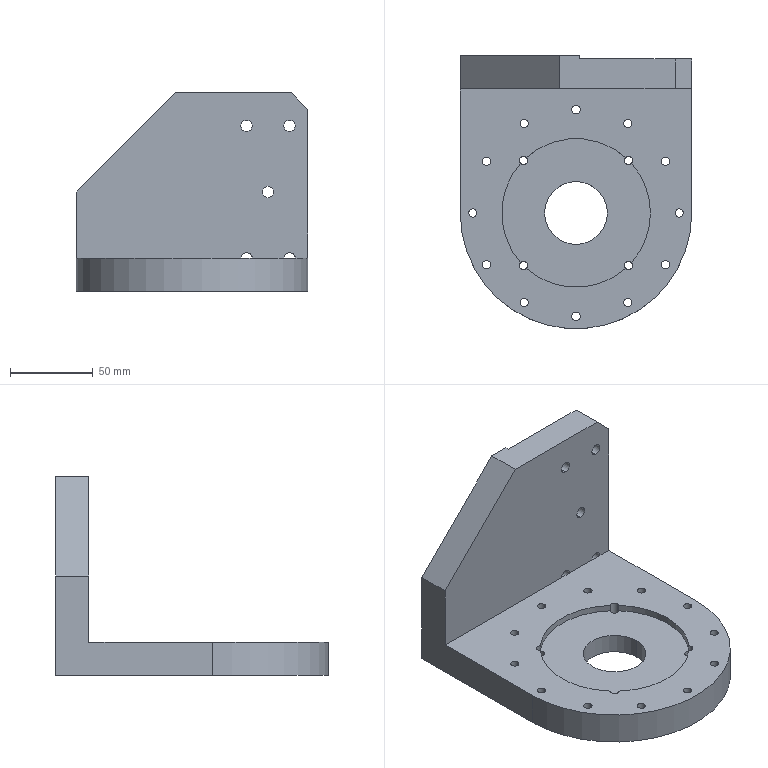Part | SolidWorks | features ICE 5, HoleWzd 3, Chamfer 2, Extrusion 1 | 1 solid | 67 faces | box 140 x 165 x 120 mm | volume 582879 mm3 | cylinder 52 | plane 15 | commonest cylinder face diameters 5 x32 6.8 x10 90 x5 38 x2 70 x2 140 x1